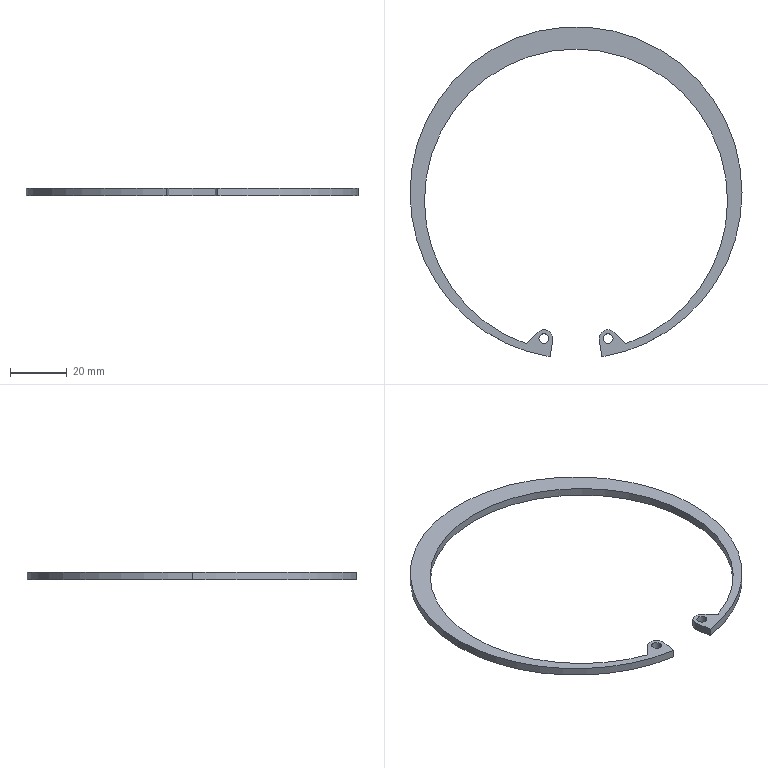Part | SolidWorks | features BaseBody 1 | 1 solid | 19 faces | box 116.7 x 115.986 x 2.8 mm | volume 5057 mm3 | cylinder 13 | plane 6 | commonest cylinder face diameters 3.5 x4 6.3 x3 106.544 x3 116.7 x3
STEP:
#1=CARTESIAN_POINT('',(-9.534,-48.506,0.));
#2=VERTEX_POINT('',#1);
#3=CARTESIAN_POINT('',(-13.034,-48.506,0.));
#4=VERTEX_POINT('',#3);
#5=CARTESIAN_POINT('',(-11.284,-48.506,0.));
#6=DIRECTION('',(0.,0.,-1.));
#7=DIRECTION('',(1.,0.,0.));
#8=AXIS2_PLACEMENT_3D('',#5,#6,#7);
#9=CIRCLE('',#8,1.75);
#10=EDGE_CURVE('',#2,#4,#9,.T.);
#11=ORIENTED_EDGE('',*,*,#10,.T.);
#12=CARTESIAN_POINT('',(-13.034,-48.506,2.8));
#13=VERTEX_POINT('',#12);
#14=CARTESIAN_POINT('',(-13.034,-48.506,-161.758));
#15=DIRECTION('',(0.,0.,1.));
#16=VECTOR('',#15,1000.);
#17=LINE('',#14,#16);
#18=EDGE_CURVE('',#4,#13,#17,.T.);
#19=ORIENTED_EDGE('',*,*,#18,.T.);
#20=CARTESIAN_POINT('',(-9.534,-48.506,2.8));
#21=VERTEX_POINT('',#20);
#22=CARTESIAN_POINT('',(-11.284,-48.506,2.8));
#23=DIRECTION('',(0.,0.,-1.));
#24=DIRECTION('',(1.,0.,0.));
#25=AXIS2_PLACEMENT_3D('',#22,#23,#24);
#26=CIRCLE('',#25,1.75);
#27=EDGE_CURVE('',#21,#13,#26,.T.);
#28=ORIENTED_EDGE('',*,*,#27,.F.);
#29=CARTESIAN_POINT('',(-9.534,-48.506,-161.758));
#30=DIRECTION('',(0.,0.,1.));
#31=VECTOR('',#30,1000.);
#32=LINE('',#29,#31);
#33=EDGE_CURVE('',#2,#21,#32,.T.);
#34=ORIENTED_EDGE('',*,*,#33,.F.);
#35=EDGE_LOOP('',(#11,#19,#28,#34));
#36=FACE_OUTER_BOUND('',#35,.T.);
#37=CARTESIAN_POINT('',(-11.284,-48.506,-161.758));
#38=DIRECTION('',(0.,0.,1.));
#39=DIRECTION('',(1.,0.,0.));
#40=AXIS2_PLACEMENT_3D('',#37,#38,#39);
#41=CYLINDRICAL_SURFACE('',#40,1.75);
#42=ADVANCED_FACE('',(#36),#41,.F.);
#43=CARTESIAN_POINT('',(13.034,-48.506,0.));
#44=VERTEX_POINT('',#43);
#45=CARTESIAN_POINT('',(9.534,-48.506,0.));
#46=VERTEX_POINT('',#45);
#47=CARTESIAN_POINT('',(11.284,-48.506,0.));
#48=DIRECTION('',(0.,0.,-1.));
#49=DIRECTION('',(1.,0.,0.));
#50=AXIS2_PLACEMENT_3D('',#47,#48,#49);
#51=CIRCLE('',#50,1.75);
#52=EDGE_CURVE('',#44,#46,#51,.T.);
#53=ORIENTED_EDGE('',*,*,#52,.T.);
#54=CARTESIAN_POINT('',(9.534,-48.506,2.8));
#55=VERTEX_POINT('',#54);
#56=CARTESIAN_POINT('',(9.534,-48.506,-161.758));
#57=DIRECTION('',(0.,0.,1.));
#58=VECTOR('',#57,1000.);
#59=LINE('',#56,#58);
#60=EDGE_CURVE('',#46,#55,#59,.T.);
#61=ORIENTED_EDGE('',*,*,#60,.T.);
#62=CARTESIAN_POINT('',(13.034,-48.506,2.8));
#63=VERTEX_POINT('',#62);
#64=CARTESIAN_POINT('',(11.284,-48.506,2.8));
#65=DIRECTION('',(0.,0.,-1.));
#66=DIRECTION('',(1.,0.,0.));
#67=AXIS2_PLACEMENT_3D('',#64,#65,#66);
#68=CIRCLE('',#67,1.75);
#69=EDGE_CURVE('',#63,#55,#68,.T.);
#70=ORIENTED_EDGE('',*,*,#69,.F.);
#71=CARTESIAN_POINT('',(13.034,-48.506,-161.758));
#72=DIRECTION('',(0.,0.,1.));
#73=VECTOR('',#72,1000.);
#74=LINE('',#71,#73);
#75=EDGE_CURVE('',#44,#63,#74,.T.);
#76=ORIENTED_EDGE('',*,*,#75,.F.);
#77=EDGE_LOOP('',(#53,#61,#70,#76));
#78=FACE_OUTER_BOUND('',#77,.T.);
#79=CARTESIAN_POINT('',(11.284,-48.506,-161.758));
#80=DIRECTION('',(0.,0.,1.));
#81=DIRECTION('',(1.,0.,0.));
#82=AXIS2_PLACEMENT_3D('',#79,#80,#81);
#83=CYLINDRICAL_SURFACE('',#82,1.75);
#84=ADVANCED_FACE('',(#78),#83,.F.);
#85=CARTESIAN_POINT('',(-17.533,-50.304,0.));
#86=VERTEX_POINT('',#85);
#87=CARTESIAN_POINT('',(-53.272,0.,0.));
#88=VERTEX_POINT('',#87);
#89=CARTESIAN_POINT('',(0.,0.,0.));
#90=DIRECTION('',(0.,0.,-1.));
#91=DIRECTION('',(1.,0.,0.));
#92=AXIS2_PLACEMENT_3D('',#89,#90,#91);
#93=CIRCLE('',#92,53.272);
#94=EDGE_CURVE('',#86,#88,#93,.T.);
#95=ORIENTED_EDGE('',*,*,#94,.T.);
#96=CARTESIAN_POINT('',(-53.272,0.,2.8));
#97=VERTEX_POINT('',#96);
#98=CARTESIAN_POINT('',(-53.272,0.,0.));
#99=DIRECTION('',(0.,0.,1.));
#100=VECTOR('',#99,1000.);
#101=LINE('',#98,#100);
#102=EDGE_CURVE('',#88,#97,#101,.T.);
#103=ORIENTED_EDGE('',*,*,#102,.T.);
#104=CARTESIAN_POINT('',(-17.533,-50.304,2.8));
#105=VERTEX_POINT('',#104);
#106=CARTESIAN_POINT('',(0.,0.,2.8));
#107=DIRECTION('',(0.,0.,-1.));
#108=DIRECTION('',(1.,0.,0.));
#109=AXIS2_PLACEMENT_3D('',#106,#107,#108);
#110=CIRCLE('',#109,53.272);
#111=EDGE_CURVE('',#105,#97,#110,.T.);
#112=ORIENTED_EDGE('',*,*,#111,.F.);
#113=CARTESIAN_POINT('',(-17.533,-50.304,0.));
#114=DIRECTION('',(0.,0.,1.));
#115=VECTOR('',#114,1000.);
#116=LINE('',#113,#115);
#117=EDGE_CURVE('',#86,#105,#116,.T.);
#118=ORIENTED_EDGE('',*,*,#117,.F.);
#119=EDGE_LOOP('',(#95,#103,#112,#118));
#120=FACE_OUTER_BOUND('',#119,.T.);
#121=CARTESIAN_POINT('',(0.,0.,0.));
#122=DIRECTION('',(0.,0.,1.));
#123=DIRECTION('',(1.,0.,0.));
#124=AXIS2_PLACEMENT_3D('',#121,#122,#123);
#125=CYLINDRICAL_SURFACE('',#124,53.272);
#126=ADVANCED_FACE('',(#120),#125,.F.);
#127=ORIENTED_EDGE('',*,*,#102,.F.);
#128=CARTESIAN_POINT('',(53.272,0.,0.));
#129=VERTEX_POINT('',#128);
#130=CARTESIAN_POINT('',(0.,0.,0.));
#131=DIRECTION('',(0.,0.,-1.));
#132=DIRECTION('',(1.,0.,0.));
#133=AXIS2_PLACEMENT_3D('',#130,#131,#132);
#134=CIRCLE('',#133,53.272);
#135=EDGE_CURVE('',#88,#129,#134,.T.);
#136=ORIENTED_EDGE('',*,*,#135,.T.);
#137=CARTESIAN_POINT('',(53.272,0.,2.8));
#138=VERTEX_POINT('',#137);
#139=CARTESIAN_POINT('',(53.272,0.,0.));
#140=DIRECTION('',(0.,0.,1.));
#141=VECTOR('',#140,1000.);
#142=LINE('',#139,#141);
#143=EDGE_CURVE('',#129,#138,#142,.T.);
#144=ORIENTED_EDGE('',*,*,#143,.T.);
#145=CARTESIAN_POINT('',(0.,0.,2.8));
#146=DIRECTION('',(0.,0.,-1.));
#147=DIRECTION('',(1.,0.,0.));
#148=AXIS2_PLACEMENT_3D('',#145,#146,#147);
#149=CIRCLE('',#148,53.272);
#150=EDGE_CURVE('',#97,#138,#149,.T.);
#151=ORIENTED_EDGE('',*,*,#150,.F.);
#152=EDGE_LOOP('',(#127,#136,#144,#151));
#153=FACE_OUTER_BOUND('',#152,.T.);
#154=CARTESIAN_POINT('',(0.,0.,0.));
#155=DIRECTION('',(0.,0.,1.));
#156=DIRECTION('',(1.,0.,0.));
#157=AXIS2_PLACEMENT_3D('',#154,#155,#156);
#158=CYLINDRICAL_SURFACE('',#157,53.272);
#159=ADVANCED_FACE('',(#153),#158,.F.);
#160=CARTESIAN_POINT('',(-8.173,-48.998,0.));
#161=VERTEX_POINT('',#160);
#162=CARTESIAN_POINT('',(-8.134,-48.506,0.));
#163=VERTEX_POINT('',#162);
#164=CARTESIAN_POINT('',(-11.284,-48.506,0.));
#165=DIRECTION('',(0.,0.,1.));
#166=DIRECTION('',(1.,0.,0.));
#167=AXIS2_PLACEMENT_3D('',#164,#165,#166);
#168=CIRCLE('',#167,3.15);
#169=EDGE_CURVE('',#161,#163,#168,.T.);
#170=ORIENTED_EDGE('',*,*,#169,.T.);
#171=CARTESIAN_POINT('',(-8.134,-48.506,2.8));
#172=VERTEX_POINT('',#171);
#173=CARTESIAN_POINT('',(-8.134,-48.506,0.));
#174=DIRECTION('',(0.,0.,1.));
#175=VECTOR('',#174,1000.);
#176=LINE('',#173,#175);
#177=EDGE_CURVE('',#163,#172,#176,.T.);
#178=ORIENTED_EDGE('',*,*,#177,.T.);
#179=CARTESIAN_POINT('',(-8.173,-48.998,2.8));
#180=VERTEX_POINT('',#179);
#181=CARTESIAN_POINT('',(-11.284,-48.506,2.8));
#182=DIRECTION('',(0.,0.,-1.));
#183=DIRECTION('',(1.,0.,0.));
#184=AXIS2_PLACEMENT_3D('',#181,#182,#183);
#185=CIRCLE('',#184,3.15);
#186=EDGE_CURVE('',#172,#180,#185,.T.);
#187=ORIENTED_EDGE('',*,*,#186,.T.);
#188=CARTESIAN_POINT('',(-8.173,-48.998,0.));
#189=DIRECTION('',(0.,0.,-1.));
#190=VECTOR('',#189,1000.);
#191=LINE('',#188,#190);
#192=EDGE_CURVE('',#180,#161,#191,.T.);
#193=ORIENTED_EDGE('',*,*,#192,.T.);
#194=EDGE_LOOP('',(#170,#178,#187,#193));
#195=FACE_OUTER_BOUND('',#194,.T.);
#196=CARTESIAN_POINT('',(-11.284,-48.506,0.));
#197=DIRECTION('',(0.,0.,1.));
#198=DIRECTION('',(1.,0.,0.));
#199=AXIS2_PLACEMENT_3D('',#196,#197,#198);
#200=CYLINDRICAL_SURFACE('',#199,3.15);
#201=ADVANCED_FACE('',(#195),#200,.T.);
#202=CARTESIAN_POINT('',(58.35,2.767,0.));
#203=VERTEX_POINT('',#202);
#204=CARTESIAN_POINT('',(-58.35,2.767,0.));
#205=VERTEX_POINT('',#204);
#206=CARTESIAN_POINT('',(0.,2.767,0.));
#207=DIRECTION('',(0.,0.,1.));
#208=DIRECTION('',(1.,0.,0.));
#209=AXIS2_PLACEMENT_3D('',#206,#207,#208);
#210=CIRCLE('',#209,58.35);
#211=EDGE_CURVE('',#203,#205,#210,.T.);
#212=ORIENTED_EDGE('',*,*,#211,.T.);
#213=CARTESIAN_POINT('',(-58.35,2.767,2.8));
#214=VERTEX_POINT('',#213);
#215=CARTESIAN_POINT('',(-58.35,2.767,0.));
#216=DIRECTION('',(0.,0.,1.));
#217=VECTOR('',#216,1000.);
#218=LINE('',#215,#217);
#219=EDGE_CURVE('',#205,#214,#218,.T.);
#220=ORIENTED_EDGE('',*,*,#219,.T.);
#221=CARTESIAN_POINT('',(58.35,2.767,2.8));
#222=VERTEX_POINT('',#221);
#223=CARTESIAN_POINT('',(0.,2.767,2.8));
#224=DIRECTION('',(0.,0.,-1.));
#225=DIRECTION('',(1.,0.,0.));
#226=AXIS2_PLACEMENT_3D('',#223,#224,#225);
#227=CIRCLE('',#226,58.35);
#228=EDGE_CURVE('',#214,#222,#227,.T.);
#229=ORIENTED_EDGE('',*,*,#228,.T.);
#230=CARTESIAN_POINT('',(58.35,2.767,0.));
#231=DIRECTION('',(0.,0.,1.));
#232=VECTOR('',#231,1000.);
#233=LINE('',#230,#232);
#234=EDGE_CURVE('',#203,#222,#233,.T.);
#235=ORIENTED_EDGE('',*,*,#234,.F.);
#236=EDGE_LOOP('',(#212,#220,#229,#235));
#237=FACE_OUTER_BOUND('',#236,.T.);
#238=CARTESIAN_POINT('',(0.,2.767,0.));
#239=DIRECTION('',(0.,0.,1.));
#240=DIRECTION('',(1.,0.,0.));
#241=AXIS2_PLACEMENT_3D('',#238,#239,#240);
#242=CYLINDRICAL_SURFACE('',#241,58.35);
#243=ADVANCED_FACE('',(#237),#242,.T.);
#244=CARTESIAN_POINT('',(9.1,-54.869,0.));
#245=VERTEX_POINT('',#244);
#246=CARTESIAN_POINT('',(0.,2.767,0.));
#247=DIRECTION('',(0.,0.,1.));
#248=DIRECTION('',(1.,0.,0.));
#249=AXIS2_PLACEMENT_3D('',#246,#247,#248);
#250=CIRCLE('',#249,58.35);
#251=EDGE_CURVE('',#245,#203,#250,.T.);
#252=ORIENTED_EDGE('',*,*,#251,.T.);
#253=ORIENTED_EDGE('',*,*,#234,.T.);
#254=CARTESIAN_POINT('',(9.1,-54.869,2.8));
#255=VERTEX_POINT('',#254);
#256=CARTESIAN_POINT('',(0.,2.767,2.8));
#257=DIRECTION('',(0.,0.,-1.));
#258=DIRECTION('',(1.,0.,0.));
#259=AXIS2_PLACEMENT_3D('',#256,#257,#258);
#260=CIRCLE('',#259,58.35);
#261=EDGE_CURVE('',#222,#255,#260,.T.);
#262=ORIENTED_EDGE('',*,*,#261,.T.);
#263=CARTESIAN_POINT('',(9.1,-54.869,0.));
#264=DIRECTION('',(0.,0.,1.));
#265=VECTOR('',#264,1000.);
#266=LINE('',#263,#265);
#267=EDGE_CURVE('',#245,#255,#266,.T.);
#268=ORIENTED_EDGE('',*,*,#267,.F.);
#269=EDGE_LOOP('',(#252,#253,#262,#268));
#270=FACE_OUTER_BOUND('',#269,.T.);
#271=CARTESIAN_POINT('',(0.,2.767,0.));
#272=DIRECTION('',(0.,0.,1.));
#273=DIRECTION('',(1.,0.,0.));
#274=AXIS2_PLACEMENT_3D('',#271,#272,#273);
#275=CYLINDRICAL_SURFACE('',#274,58.35);
#276=ADVANCED_FACE('',(#270),#275,.T.);
#277=ORIENTED_EDGE('',*,*,#10,.F.);
#278=CARTESIAN_POINT('',(-11.284,-48.506,0.));
#279=DIRECTION('',(0.,0.,-1.));
#280=DIRECTION('',(1.,0.,0.));
#281=AXIS2_PLACEMENT_3D('',#278,#279,#280);
#282=CIRCLE('',#281,1.75);
#283=EDGE_CURVE('',#4,#2,#282,.T.);
#284=ORIENTED_EDGE('',*,*,#283,.F.);
#285=EDGE_LOOP('',(#277,#284));
#286=FACE_BOUND('',#285,.T.);
#287=ORIENTED_EDGE('',*,*,#52,.F.);
#288=CARTESIAN_POINT('',(11.284,-48.506,0.));
#289=DIRECTION('',(0.,0.,-1.));
#290=DIRECTION('',(1.,0.,0.));
#291=AXIS2_PLACEMENT_3D('',#288,#289,#290);
#292=CIRCLE('',#291,1.75);
#293=EDGE_CURVE('',#46,#44,#292,.T.);
#294=ORIENTED_EDGE('',*,*,#293,.F.);
#295=EDGE_LOOP('',(#287,#294));
#296=FACE_BOUND('',#295,.T.);
#297=CARTESIAN_POINT('',(13.513,-46.28,0.));
#298=VERTEX_POINT('',#297);
#299=CARTESIAN_POINT('',(8.173,-48.998,0.));
#300=VERTEX_POINT('',#299);
#301=CARTESIAN_POINT('',(11.284,-48.506,0.));
#302=DIRECTION('',(0.,0.,1.));
#303=DIRECTION('',(1.,0.,0.));
#304=AXIS2_PLACEMENT_3D('',#301,#302,#303);
#305=CIRCLE('',#304,3.15);
#306=EDGE_CURVE('',#298,#300,#305,.T.);
#307=ORIENTED_EDGE('',*,*,#306,.F.);
#308=CARTESIAN_POINT('',(17.533,-50.304,0.));
#309=VERTEX_POINT('',#308);
#310=CARTESIAN_POINT('',(17.533,-50.304,0.));
#311=DIRECTION('',(-0.7068,0.7074,0.));
#312=VECTOR('',#311,1000.);
#313=LINE('',#310,#312);
#314=EDGE_CURVE('',#309,#298,#313,.T.);
#315=ORIENTED_EDGE('',*,*,#314,.F.);
#316=CARTESIAN_POINT('',(0.,0.,0.));
#317=DIRECTION('',(0.,0.,-1.));
#318=DIRECTION('',(1.,0.,0.));
#319=AXIS2_PLACEMENT_3D('',#316,#317,#318);
#320=CIRCLE('',#319,53.272);
#321=EDGE_CURVE('',#129,#309,#320,.T.);
#322=ORIENTED_EDGE('',*,*,#321,.F.);
#323=ORIENTED_EDGE('',*,*,#135,.F.);
#324=ORIENTED_EDGE('',*,*,#94,.F.);
#325=CARTESIAN_POINT('',(-13.513,-46.28,0.));
#326=VERTEX_POINT('',#325);
#327=CARTESIAN_POINT('',(-13.513,-46.28,0.));
#328=DIRECTION('',(-0.7068,-0.7074,0.));
#329=VECTOR('',#328,1000.);
#330=LINE('',#327,#329);
#331=EDGE_CURVE('',#326,#86,#330,.T.);
#332=ORIENTED_EDGE('',*,*,#331,.F.);
#333=CARTESIAN_POINT('',(-11.284,-48.506,0.));
#334=DIRECTION('',(0.,0.,1.));
#335=DIRECTION('',(1.,0.,0.));
#336=AXIS2_PLACEMENT_3D('',#333,#334,#335);
#337=CIRCLE('',#336,3.15);
#338=EDGE_CURVE('',#163,#326,#337,.T.);
#339=ORIENTED_EDGE('',*,*,#338,.F.);
#340=ORIENTED_EDGE('',*,*,#169,.F.);
#341=CARTESIAN_POINT('',(-9.1,-54.869,0.));
#342=VERTEX_POINT('',#341);
#343=CARTESIAN_POINT('',(-9.1,-54.869,0.));
#344=DIRECTION('',(0.156,0.9878,0.));
#345=VECTOR('',#344,1000.);
#346=LINE('',#343,#345);
#347=EDGE_CURVE('',#342,#161,#346,.T.);
#348=ORIENTED_EDGE('',*,*,#347,.F.);
#349=CARTESIAN_POINT('',(0.,2.767,0.));
#350=DIRECTION('',(0.,0.,1.));
#351=DIRECTION('',(1.,0.,0.));
#352=AXIS2_PLACEMENT_3D('',#349,#350,#351);
#353=CIRCLE('',#352,58.35);
#354=EDGE_CURVE('',#205,#342,#353,.T.);
#355=ORIENTED_EDGE('',*,*,#354,.F.);
#356=ORIENTED_EDGE('',*,*,#211,.F.);
#357=ORIENTED_EDGE('',*,*,#251,.F.);
#358=CARTESIAN_POINT('',(8.173,-48.998,0.));
#359=DIRECTION('',(0.156,-0.9878,0.));
#360=VECTOR('',#359,1000.);
#361=LINE('',#358,#360);
#362=EDGE_CURVE('',#300,#245,#361,.T.);
#363=ORIENTED_EDGE('',*,*,#362,.F.);
#364=EDGE_LOOP('',(#307,#315,#322,#323,#324,#332,#339,#340,#348,#355,#356,#357,#363));
#365=FACE_OUTER_BOUND('',#364,.T.);
#366=CARTESIAN_POINT('',(0.,-2.246,0.));
#367=DIRECTION('',(0.,0.,1.));
#368=DIRECTION('',(1.,0.,0.));
#369=AXIS2_PLACEMENT_3D('',#366,#367,#368);
#370=PLANE('',#369);
#371=ADVANCED_FACE('',(#286,#296,#365),#370,.F.);
#372=ORIENTED_EDGE('',*,*,#18,.F.);
#373=ORIENTED_EDGE('',*,*,#283,.T.);
#374=ORIENTED_EDGE('',*,*,#33,.T.);
#375=CARTESIAN_POINT('',(-11.284,-48.506,2.8));
#376=DIRECTION('',(0.,0.,-1.));
#377=DIRECTION('',(1.,0.,0.));
#378=AXIS2_PLACEMENT_3D('',#375,#376,#377);
#379=CIRCLE('',#378,1.75);
#380=EDGE_CURVE('',#13,#21,#379,.T.);
#381=ORIENTED_EDGE('',*,*,#380,.F.);
#382=EDGE_LOOP('',(#372,#373,#374,#381));
#383=FACE_OUTER_BOUND('',#382,.T.);
#384=CARTESIAN_POINT('',(-11.284,-48.506,-161.758));
#385=DIRECTION('',(0.,0.,1.));
#386=DIRECTION('',(1.,0.,0.));
#387=AXIS2_PLACEMENT_3D('',#384,#385,#386);
#388=CYLINDRICAL_SURFACE('',#387,1.75);
#389=ADVANCED_FACE('',(#383),#388,.F.);
#390=ORIENTED_EDGE('',*,*,#60,.F.);
#391=ORIENTED_EDGE('',*,*,#293,.T.);
#392=ORIENTED_EDGE('',*,*,#75,.T.);
#393=CARTESIAN_POINT('',(11.284,-48.506,2.8));
#394=DIRECTION('',(0.,0.,-1.));
#395=DIRECTION('',(1.,0.,0.));
#396=AXIS2_PLACEMENT_3D('',#393,#394,#395);
#397=CIRCLE('',#396,1.75);
#398=EDGE_CURVE('',#55,#63,#397,.T.);
#399=ORIENTED_EDGE('',*,*,#398,.F.);
#400=EDGE_LOOP('',(#390,#391,#392,#399));
#401=FACE_OUTER_BOUND('',#400,.T.);
#402=CARTESIAN_POINT('',(11.284,-48.506,-161.758));
#403=DIRECTION('',(0.,0.,1.));
#404=DIRECTION('',(1.,0.,0.));
#405=AXIS2_PLACEMENT_3D('',#402,#403,#404);
#406=CYLINDRICAL_SURFACE('',#405,1.75);
#407=ADVANCED_FACE('',(#401),#406,.F.);
#408=ORIENTED_EDGE('',*,*,#362,.T.);
#409=ORIENTED_EDGE('',*,*,#267,.T.);
#410=CARTESIAN_POINT('',(8.173,-48.998,2.8));
#411=VERTEX_POINT('',#410);
#412=CARTESIAN_POINT('',(9.1,-54.869,2.8));
#413=DIRECTION('',(-0.156,0.9878,0.));
#414=VECTOR('',#413,1000.);
#415=LINE('',#412,#414);
#416=EDGE_CURVE('',#255,#411,#415,.T.);
#417=ORIENTED_EDGE('',*,*,#416,.T.);
#418=CARTESIAN_POINT('',(8.173,-48.998,0.));
#419=DIRECTION('',(0.,0.,-1.));
#420=VECTOR('',#419,1000.);
#421=LINE('',#418,#420);
#422=EDGE_CURVE('',#411,#300,#421,.T.);
#423=ORIENTED_EDGE('',*,*,#422,.T.);
#424=EDGE_LOOP('',(#408,#409,#417,#423));
#425=FACE_OUTER_BOUND('',#424,.T.);
#426=CARTESIAN_POINT('',(9.1,-54.869,0.));
#427=DIRECTION('',(-0.9878,-0.156,0.));
#428=DIRECTION('',(0.156,-0.9878,0.));
#429=AXIS2_PLACEMENT_3D('',#426,#427,#428);
#430=PLANE('',#429);
#431=ADVANCED_FACE('',(#425),#430,.T.);
#432=ORIENTED_EDGE('',*,*,#306,.T.);
#433=ORIENTED_EDGE('',*,*,#422,.F.);
#434=CARTESIAN_POINT('',(13.513,-46.28,2.8));
#435=VERTEX_POINT('',#434);
#436=CARTESIAN_POINT('',(11.284,-48.506,2.8));
#437=DIRECTION('',(0.,0.,-1.));
#438=DIRECTION('',(1.,0.,0.));
#439=AXIS2_PLACEMENT_3D('',#436,#437,#438);
#440=CIRCLE('',#439,3.15);
#441=EDGE_CURVE('',#411,#435,#440,.T.);
#442=ORIENTED_EDGE('',*,*,#441,.T.);
#443=CARTESIAN_POINT('',(13.513,-46.28,0.));
#444=DIRECTION('',(0.,0.,-1.));
#445=VECTOR('',#444,1000.);
#446=LINE('',#443,#445);
#447=EDGE_CURVE('',#435,#298,#446,.T.);
#448=ORIENTED_EDGE('',*,*,#447,.T.);
#449=EDGE_LOOP('',(#432,#433,#442,#448));
#450=FACE_OUTER_BOUND('',#449,.T.);
#451=CARTESIAN_POINT('',(11.284,-48.506,0.));
#452=DIRECTION('',(0.,0.,1.));
#453=DIRECTION('',(1.,0.,0.));
#454=AXIS2_PLACEMENT_3D('',#451,#452,#453);
#455=CYLINDRICAL_SURFACE('',#454,3.15);
#456=ADVANCED_FACE('',(#450),#455,.T.);
#457=ORIENTED_EDGE('',*,*,#314,.T.);
#458=ORIENTED_EDGE('',*,*,#447,.F.);
#459=CARTESIAN_POINT('',(17.533,-50.304,2.8));
#460=VERTEX_POINT('',#459);
#461=CARTESIAN_POINT('',(13.513,-46.28,2.8));
#462=DIRECTION('',(0.7068,-0.7074,0.));
#463=VECTOR('',#462,1000.);
#464=LINE('',#461,#463);
#465=EDGE_CURVE('',#435,#460,#464,.T.);
#466=ORIENTED_EDGE('',*,*,#465,.T.);
#467=CARTESIAN_POINT('',(17.533,-50.304,0.));
#468=DIRECTION('',(0.,0.,-1.));
#469=VECTOR('',#468,1000.);
#470=LINE('',#467,#469);
#471=EDGE_CURVE('',#460,#309,#470,.T.);
#472=ORIENTED_EDGE('',*,*,#471,.T.);
#473=EDGE_LOOP('',(#457,#458,#466,#472));
#474=FACE_OUTER_BOUND('',#473,.T.);
#475=CARTESIAN_POINT('',(13.513,-46.28,0.));
#476=DIRECTION('',(0.7074,0.7068,0.));
#477=DIRECTION('',(-0.7068,0.7074,0.));
#478=AXIS2_PLACEMENT_3D('',#475,#476,#477);
#479=PLANE('',#478);
#480=ADVANCED_FACE('',(#474),#479,.T.);
#481=ORIENTED_EDGE('',*,*,#143,.F.);
#482=ORIENTED_EDGE('',*,*,#321,.T.);
#483=ORIENTED_EDGE('',*,*,#471,.F.);
#484=CARTESIAN_POINT('',(0.,0.,2.8));
#485=DIRECTION('',(0.,0.,-1.));
#486=DIRECTION('',(1.,0.,0.));
#487=AXIS2_PLACEMENT_3D('',#484,#485,#486);
#488=CIRCLE('',#487,53.272);
#489=EDGE_CURVE('',#138,#460,#488,.T.);
#490=ORIENTED_EDGE('',*,*,#489,.F.);
#491=EDGE_LOOP('',(#481,#482,#483,#490));
#492=FACE_OUTER_BOUND('',#491,.T.);
#493=CARTESIAN_POINT('',(0.,0.,0.));
#494=DIRECTION('',(0.,0.,1.));
#495=DIRECTION('',(1.,0.,0.));
#496=AXIS2_PLACEMENT_3D('',#493,#494,#495);
#497=CYLINDRICAL_SURFACE('',#496,53.272);
#498=ADVANCED_FACE('',(#492),#497,.F.);
#499=ORIENTED_EDGE('',*,*,#331,.T.);
#500=ORIENTED_EDGE('',*,*,#117,.T.);
#501=CARTESIAN_POINT('',(-13.513,-46.28,2.8));
#502=VERTEX_POINT('',#501);
#503=CARTESIAN_POINT('',(-17.533,-50.304,2.8));
#504=DIRECTION('',(0.7068,0.7074,0.));
#505=VECTOR('',#504,1000.);
#506=LINE('',#503,#505);
#507=EDGE_CURVE('',#105,#502,#506,.T.);
#508=ORIENTED_EDGE('',*,*,#507,.T.);
#509=CARTESIAN_POINT('',(-13.513,-46.28,0.));
#510=DIRECTION('',(0.,0.,-1.));
#511=VECTOR('',#510,1000.);
#512=LINE('',#509,#511);
#513=EDGE_CURVE('',#502,#326,#512,.T.);
#514=ORIENTED_EDGE('',*,*,#513,.T.);
#515=EDGE_LOOP('',(#499,#500,#508,#514));
#516=FACE_OUTER_BOUND('',#515,.T.);
#517=CARTESIAN_POINT('',(-17.533,-50.304,0.));
#518=DIRECTION('',(-0.7074,0.7068,0.));
#519=DIRECTION('',(-0.7068,-0.7074,0.));
#520=AXIS2_PLACEMENT_3D('',#517,#518,#519);
#521=PLANE('',#520);
#522=ADVANCED_FACE('',(#516),#521,.T.);
#523=ORIENTED_EDGE('',*,*,#177,.F.);
#524=ORIENTED_EDGE('',*,*,#338,.T.);
#525=ORIENTED_EDGE('',*,*,#513,.F.);
#526=CARTESIAN_POINT('',(-11.284,-48.506,2.8));
#527=DIRECTION('',(0.,0.,-1.));
#528=DIRECTION('',(1.,0.,0.));
#529=AXIS2_PLACEMENT_3D('',#526,#527,#528);
#530=CIRCLE('',#529,3.15);
#531=EDGE_CURVE('',#502,#172,#530,.T.);
#532=ORIENTED_EDGE('',*,*,#531,.T.);
#533=EDGE_LOOP('',(#523,#524,#525,#532));
#534=FACE_OUTER_BOUND('',#533,.T.);
#535=CARTESIAN_POINT('',(-11.284,-48.506,0.));
#536=DIRECTION('',(0.,0.,1.));
#537=DIRECTION('',(1.,0.,0.));
#538=AXIS2_PLACEMENT_3D('',#535,#536,#537);
#539=CYLINDRICAL_SURFACE('',#538,3.15);
#540=ADVANCED_FACE('',(#534),#539,.T.);
#541=ORIENTED_EDGE('',*,*,#347,.T.);
#542=ORIENTED_EDGE('',*,*,#192,.F.);
#543=CARTESIAN_POINT('',(-9.1,-54.869,2.8));
#544=VERTEX_POINT('',#543);
#545=CARTESIAN_POINT('',(-8.173,-48.998,2.8));
#546=DIRECTION('',(-0.156,-0.9878,0.));
#547=VECTOR('',#546,1000.);
#548=LINE('',#545,#547);
#549=EDGE_CURVE('',#180,#544,#548,.T.);
#550=ORIENTED_EDGE('',*,*,#549,.T.);
#551=CARTESIAN_POINT('',(-9.1,-54.869,0.));
#552=DIRECTION('',(0.,0.,-1.));
#553=VECTOR('',#552,1000.);
#554=LINE('',#551,#553);
#555=EDGE_CURVE('',#544,#342,#554,.T.);
#556=ORIENTED_EDGE('',*,*,#555,.T.);
#557=EDGE_LOOP('',(#541,#542,#550,#556));
#558=FACE_OUTER_BOUND('',#557,.T.);
#559=CARTESIAN_POINT('',(-8.173,-48.998,0.));
#560=DIRECTION('',(0.9878,-0.156,0.));
#561=DIRECTION('',(0.156,0.9878,0.));
#562=AXIS2_PLACEMENT_3D('',#559,#560,#561);
#563=PLANE('',#562);
#564=ADVANCED_FACE('',(#558),#563,.T.);
#565=ORIENTED_EDGE('',*,*,#219,.F.);
#566=ORIENTED_EDGE('',*,*,#354,.T.);
#567=ORIENTED_EDGE('',*,*,#555,.F.);
#568=CARTESIAN_POINT('',(0.,2.767,2.8));
#569=DIRECTION('',(0.,0.,-1.));
#570=DIRECTION('',(1.,0.,0.));
#571=AXIS2_PLACEMENT_3D('',#568,#569,#570);
#572=CIRCLE('',#571,58.35);
#573=EDGE_CURVE('',#544,#214,#572,.T.);
#574=ORIENTED_EDGE('',*,*,#573,.T.);
#575=EDGE_LOOP('',(#565,#566,#567,#574));
#576=FACE_OUTER_BOUND('',#575,.T.);
#577=CARTESIAN_POINT('',(0.,2.767,0.));
#578=DIRECTION('',(0.,0.,1.));
#579=DIRECTION('',(1.,0.,0.));
#580=AXIS2_PLACEMENT_3D('',#577,#578,#579);
#581=CYLINDRICAL_SURFACE('',#580,58.35);
#582=ADVANCED_FACE('',(#576),#581,.T.);
#583=ORIENTED_EDGE('',*,*,#27,.T.);
#584=ORIENTED_EDGE('',*,*,#380,.T.);
#585=EDGE_LOOP('',(#583,#584));
#586=FACE_BOUND('',#585,.T.);
#587=ORIENTED_EDGE('',*,*,#69,.T.);
#588=ORIENTED_EDGE('',*,*,#398,.T.);
#589=EDGE_LOOP('',(#587,#588));
#590=FACE_BOUND('',#589,.T.);
#591=ORIENTED_EDGE('',*,*,#111,.T.);
#592=ORIENTED_EDGE('',*,*,#150,.T.);
#593=ORIENTED_EDGE('',*,*,#489,.T.);
#594=ORIENTED_EDGE('',*,*,#465,.F.);
#595=ORIENTED_EDGE('',*,*,#441,.F.);
#596=ORIENTED_EDGE('',*,*,#416,.F.);
#597=ORIENTED_EDGE('',*,*,#261,.F.);
#598=ORIENTED_EDGE('',*,*,#228,.F.);
#599=ORIENTED_EDGE('',*,*,#573,.F.);
#600=ORIENTED_EDGE('',*,*,#549,.F.);
#601=ORIENTED_EDGE('',*,*,#186,.F.);
#602=ORIENTED_EDGE('',*,*,#531,.F.);
#603=ORIENTED_EDGE('',*,*,#507,.F.);
#604=EDGE_LOOP('',(#591,#592,#593,#594,#595,#596,#597,#598,#599,#600,#601,#602,#603));
#605=FACE_OUTER_BOUND('',#604,.T.);
#606=CARTESIAN_POINT('',(0.,-2.246,2.8));
#607=DIRECTION('',(0.,0.,1.));
#608=DIRECTION('',(1.,0.,0.));
#609=AXIS2_PLACEMENT_3D('',#606,#607,#608);
#610=PLANE('',#609);
#611=ADVANCED_FACE('',(#586,#590,#605),#610,.T.);
#612=CLOSED_SHELL('',(#42,#84,#126,#159,#201,#243,#276,#371,#389,#407,#431,#456,#480,#498,#522,#540,#564,#582,#611));
#613=MANIFOLD_SOLID_BREP('',#612);
#614=CARTESIAN_POINT('',(0.,0.,0.));
#615=DIRECTION('',(0.,0.,1.));
#616=DIRECTION('',(1.,0.,0.));
#617=AXIS2_PLACEMENT_3D('',#614,#615,#616);
#618=(LENGTH_UNIT()NAMED_UNIT(*)SI_UNIT(.MILLI.,.METRE.));
#619=UNCERTAINTY_MEASURE_WITH_UNIT(LENGTH_MEASURE(0.00001),#618,'','');
#620=(NAMED_UNIT(*)PLANE_ANGLE_UNIT()SI_UNIT($,.RADIAN.));
#621=(NAMED_UNIT(*)SI_UNIT($,.STERADIAN.)SOLID_ANGLE_UNIT());
#622=(GEOMETRIC_REPRESENTATION_CONTEXT(3)GLOBAL_UNCERTAINTY_ASSIGNED_CONTEXT((#619))GLOBAL_UNIT_ASSIGNED_CONTEXT((#618,#620,#621))REPRESENTATION_CONTEXT('',''));
#623=ADVANCED_BREP_SHAPE_REPRESENTATION('',(#613,#617),#622);